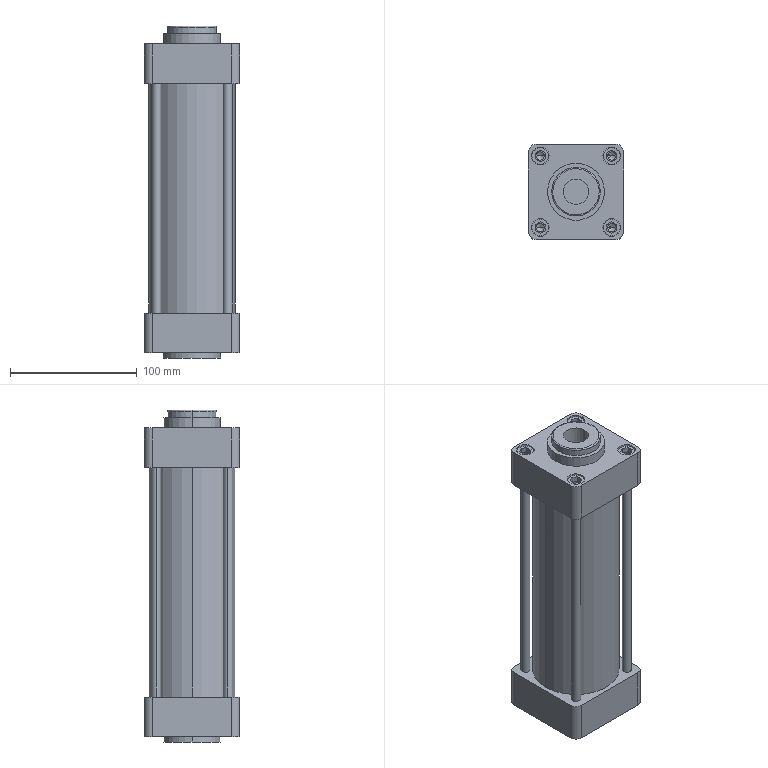Part | SolidWorks | features BaseBody 1 | 1 solid | 229 faces | box 75 x 75 x 262 mm | volume 538343 mm3 | plane 111 | cylinder 84 | cone 32 | spline 2 | commonest cylinder face diameters 6.647 x16 13 x16 14 x16 7.2 x8 12 x8 9.8 x4